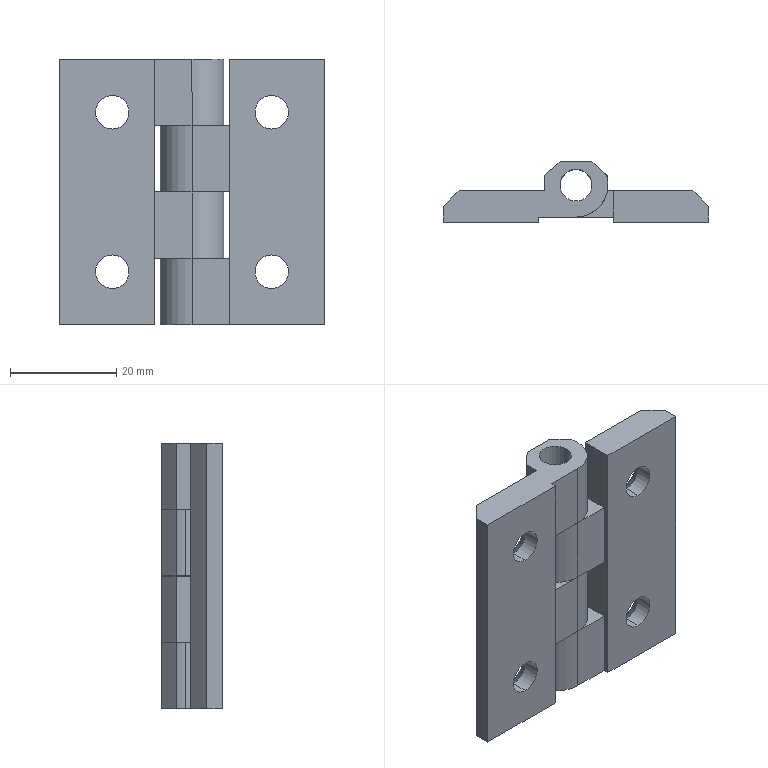Part | SolidWorks | 2 solids | 72 faces | box 50 x 11.5 x 50 mm | volume 13478 mm3 | plane 40 | cylinder 24 | cone 8 | commonest cylinder face diameters 6 x8 6.3 x8 12 x8